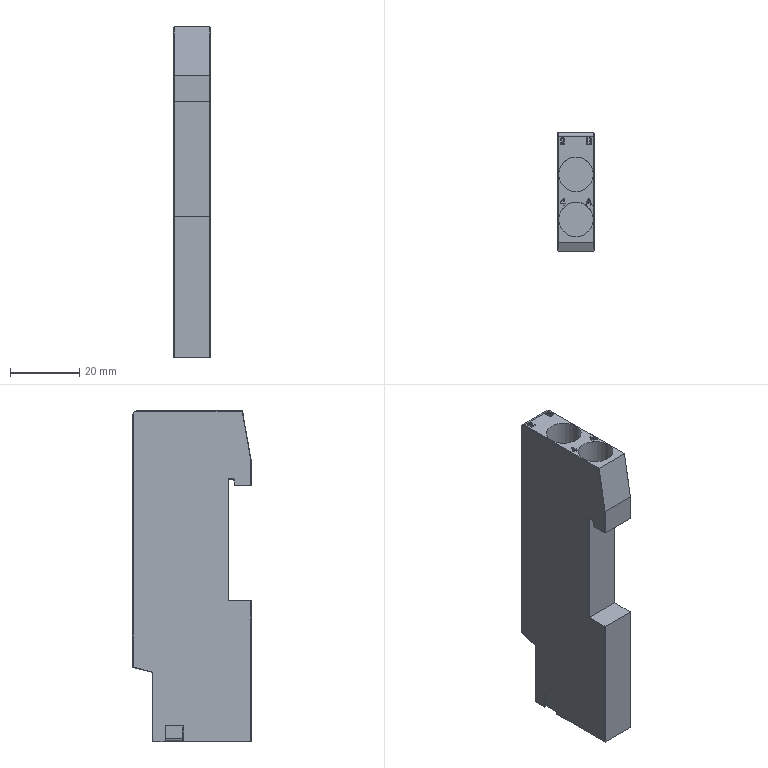Part | STEP file | SS5V1-16S3AD-08B-N1_Valve Base | 1 solid | 149 faces | box 10.5 x 34 x 95.55 mm | volume 27614 mm3 | plane 120 | spline 16 | cylinder 11 | cone 2 | commonest cylinder face diameters 1.8 x4 10 x4 0.5 x1 1.5 x1 2 x1